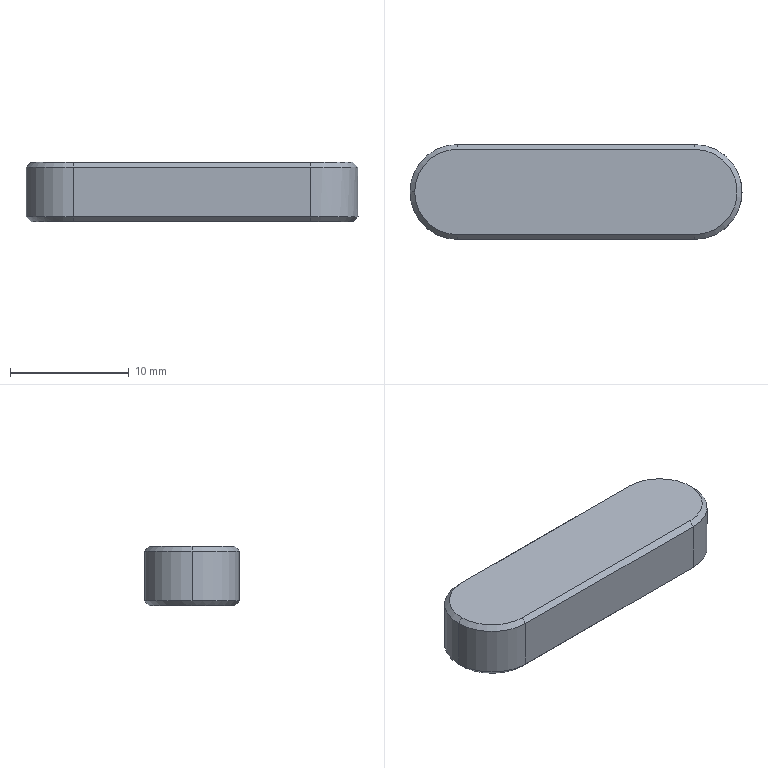Part | SolidWorks | features BaseBody 1 | 1 solid | 17 faces | box 28 x 8 x 5 mm | volume 1041 mm3 | plane 8 | cone 6 | cylinder 3 | commonest cylinder face diameters 8 x3
STEP:
#1=CARTESIAN_POINT('',(24.,-3.6,-3.));
#2=VERTEX_POINT('',#1);
#3=CARTESIAN_POINT('',(27.6,0.,-3.));
#4=VERTEX_POINT('',#3);
#5=CARTESIAN_POINT('',(24.,0.,-3.));
#6=DIRECTION('',(0.,0.,1.));
#7=DIRECTION('',(1.,0.,0.));
#8=AXIS2_PLACEMENT_3D('',#5,#6,#7);
#9=CIRCLE('',#8,3.6);
#10=EDGE_CURVE('',#2,#4,#9,.T.);
#11=ORIENTED_EDGE('',*,*,#10,.T.);
#12=CARTESIAN_POINT('',(28.,0.,-2.6));
#13=VERTEX_POINT('',#12);
#14=CARTESIAN_POINT('',(28.,0.,-2.6));
#15=DIRECTION('',(0.7071,0.,0.7071));
#16=VECTOR('',#15,1000.);
#17=LINE('',#14,#16);
#18=EDGE_CURVE('',#4,#13,#17,.T.);
#19=ORIENTED_EDGE('',*,*,#18,.T.);
#20=CARTESIAN_POINT('',(24.,-4.,-2.6));
#21=VERTEX_POINT('',#20);
#22=CARTESIAN_POINT('',(24.,0.,-2.6));
#23=DIRECTION('',(0.,0.,-1.));
#24=DIRECTION('',(0.,1.,0.));
#25=AXIS2_PLACEMENT_3D('',#22,#23,#24);
#26=CIRCLE('',#25,4.);
#27=EDGE_CURVE('',#13,#21,#26,.T.);
#28=ORIENTED_EDGE('',*,*,#27,.T.);
#29=CARTESIAN_POINT('',(24.,-3.8,-2.8));
#30=DIRECTION('',(0.,-0.7071,0.7071));
#31=VECTOR('',#30,1000.);
#32=LINE('',#29,#31);
#33=EDGE_CURVE('',#2,#21,#32,.T.);
#34=ORIENTED_EDGE('',*,*,#33,.F.);
#35=EDGE_LOOP('',(#11,#19,#28,#34));
#36=FACE_OUTER_BOUND('',#35,.T.);
#37=CARTESIAN_POINT('',(24.,0.,-2.6));
#38=DIRECTION('',(0.,0.,1.));
#39=DIRECTION('',(1.,0.,0.));
#40=AXIS2_PLACEMENT_3D('',#37,#38,#39);
#41=CONICAL_SURFACE('',#40,4.,0.7854);
#42=ADVANCED_FACE('',(#36),#41,.T.);
#43=CARTESIAN_POINT('',(4.,-4.,1.6));
#44=VERTEX_POINT('',#43);
#45=CARTESIAN_POINT('',(0.,0.,1.6));
#46=VERTEX_POINT('',#45);
#47=CARTESIAN_POINT('',(4.,0.,1.6));
#48=DIRECTION('',(0.,0.,-1.));
#49=DIRECTION('',(-1.,0.,0.));
#50=AXIS2_PLACEMENT_3D('',#47,#48,#49);
#51=CIRCLE('',#50,4.);
#52=EDGE_CURVE('',#44,#46,#51,.T.);
#53=ORIENTED_EDGE('',*,*,#52,.T.);
#54=CARTESIAN_POINT('',(0.,0.,-2.6));
#55=VERTEX_POINT('',#54);
#56=CARTESIAN_POINT('',(0.,0.,0.));
#57=DIRECTION('',(0.,0.,-1.));
#58=VECTOR('',#57,1000.);
#59=LINE('',#56,#58);
#60=EDGE_CURVE('',#46,#55,#59,.T.);
#61=ORIENTED_EDGE('',*,*,#60,.T.);
#62=CARTESIAN_POINT('',(4.,-4.,-2.6));
#63=VERTEX_POINT('',#62);
#64=CARTESIAN_POINT('',(4.,0.,-2.6));
#65=DIRECTION('',(0.,0.,-1.));
#66=DIRECTION('',(0.,-1.,0.));
#67=AXIS2_PLACEMENT_3D('',#64,#65,#66);
#68=CIRCLE('',#67,4.);
#69=EDGE_CURVE('',#63,#55,#68,.T.);
#70=ORIENTED_EDGE('',*,*,#69,.F.);
#71=CARTESIAN_POINT('',(4.,-4.,0.));
#72=DIRECTION('',(0.,0.,-1.));
#73=VECTOR('',#72,1000.);
#74=LINE('',#71,#73);
#75=EDGE_CURVE('',#44,#63,#74,.T.);
#76=ORIENTED_EDGE('',*,*,#75,.F.);
#77=EDGE_LOOP('',(#53,#61,#70,#76));
#78=FACE_OUTER_BOUND('',#77,.T.);
#79=CARTESIAN_POINT('',(4.,0.,0.));
#80=DIRECTION('',(0.,0.,-1.));
#81=DIRECTION('',(-1.,0.,0.));
#82=AXIS2_PLACEMENT_3D('',#79,#80,#81);
#83=CYLINDRICAL_SURFACE('',#82,4.);
#84=ADVANCED_FACE('',(#78),#83,.T.);
#85=CARTESIAN_POINT('',(4.,-3.6,2.));
#86=VERTEX_POINT('',#85);
#87=CARTESIAN_POINT('',(0.4,0.,2.));
#88=VERTEX_POINT('',#87);
#89=CARTESIAN_POINT('',(4.,0.,2.));
#90=DIRECTION('',(0.,0.,-1.));
#91=DIRECTION('',(-1.,0.,0.));
#92=AXIS2_PLACEMENT_3D('',#89,#90,#91);
#93=CIRCLE('',#92,3.6);
#94=EDGE_CURVE('',#86,#88,#93,.T.);
#95=ORIENTED_EDGE('',*,*,#94,.T.);
#96=CARTESIAN_POINT('',(0.,0.,1.6));
#97=DIRECTION('',(-0.7071,0.,-0.7071));
#98=VECTOR('',#97,1000.);
#99=LINE('',#96,#98);
#100=EDGE_CURVE('',#88,#46,#99,.T.);
#101=ORIENTED_EDGE('',*,*,#100,.T.);
#102=ORIENTED_EDGE('',*,*,#52,.F.);
#103=CARTESIAN_POINT('',(4.,-3.8,1.8));
#104=DIRECTION('',(0.,-0.7071,-0.7071));
#105=VECTOR('',#104,1000.);
#106=LINE('',#103,#105);
#107=EDGE_CURVE('',#86,#44,#106,.T.);
#108=ORIENTED_EDGE('',*,*,#107,.F.);
#109=EDGE_LOOP('',(#95,#101,#102,#108));
#110=FACE_OUTER_BOUND('',#109,.T.);
#111=CARTESIAN_POINT('',(4.,0.,1.6));
#112=DIRECTION('',(0.,0.,-1.));
#113=DIRECTION('',(-1.,0.,0.));
#114=AXIS2_PLACEMENT_3D('',#111,#112,#113);
#115=CONICAL_SURFACE('',#114,4.,0.7854);
#116=ADVANCED_FACE('',(#110),#115,.T.);
#117=CARTESIAN_POINT('',(4.,3.6,-3.));
#118=VERTEX_POINT('',#117);
#119=CARTESIAN_POINT('',(4.,-3.6,-3.));
#120=VERTEX_POINT('',#119);
#121=CARTESIAN_POINT('',(4.,0.,-3.));
#122=DIRECTION('',(0.,0.,1.));
#123=DIRECTION('',(1.,0.,0.));
#124=AXIS2_PLACEMENT_3D('',#121,#122,#123);
#125=CIRCLE('',#124,3.6);
#126=EDGE_CURVE('',#118,#120,#125,.T.);
#127=ORIENTED_EDGE('',*,*,#126,.F.);
#128=CARTESIAN_POINT('',(24.,3.6,-3.));
#129=VERTEX_POINT('',#128);
#130=CARTESIAN_POINT('',(14.,3.6,-3.));
#131=DIRECTION('',(-1.,0.,0.));
#132=VECTOR('',#131,1000.);
#133=LINE('',#130,#132);
#134=EDGE_CURVE('',#129,#118,#133,.T.);
#135=ORIENTED_EDGE('',*,*,#134,.F.);
#136=CARTESIAN_POINT('',(24.,0.,-3.));
#137=DIRECTION('',(0.,0.,1.));
#138=DIRECTION('',(1.,0.,0.));
#139=AXIS2_PLACEMENT_3D('',#136,#137,#138);
#140=CIRCLE('',#139,3.6);
#141=EDGE_CURVE('',#4,#129,#140,.T.);
#142=ORIENTED_EDGE('',*,*,#141,.F.);
#143=ORIENTED_EDGE('',*,*,#10,.F.);
#144=CARTESIAN_POINT('',(14.,-3.6,-3.));
#145=DIRECTION('',(1.,0.,0.));
#146=VECTOR('',#145,1000.);
#147=LINE('',#144,#146);
#148=EDGE_CURVE('',#120,#2,#147,.T.);
#149=ORIENTED_EDGE('',*,*,#148,.F.);
#150=EDGE_LOOP('',(#127,#135,#142,#143,#149));
#151=FACE_OUTER_BOUND('',#150,.T.);
#152=CARTESIAN_POINT('',(14.,0.,-3.));
#153=DIRECTION('',(0.,0.,1.));
#154=DIRECTION('',(1.,0.,0.));
#155=AXIS2_PLACEMENT_3D('',#152,#153,#154);
#156=PLANE('',#155);
#157=ADVANCED_FACE('',(#151),#156,.F.);
#158=CARTESIAN_POINT('',(4.,-3.8,-2.8));
#159=DIRECTION('',(0.,0.7071,-0.7071));
#160=VECTOR('',#159,1000.);
#161=LINE('',#158,#160);
#162=EDGE_CURVE('',#63,#120,#161,.T.);
#163=ORIENTED_EDGE('',*,*,#162,.T.);
#164=ORIENTED_EDGE('',*,*,#148,.T.);
#165=ORIENTED_EDGE('',*,*,#33,.T.);
#166=CARTESIAN_POINT('',(9.,-4.,-2.6));
#167=DIRECTION('',(-1.,0.,0.));
#168=VECTOR('',#167,1000.);
#169=LINE('',#166,#168);
#170=EDGE_CURVE('',#21,#63,#169,.T.);
#171=ORIENTED_EDGE('',*,*,#170,.T.);
#172=EDGE_LOOP('',(#163,#164,#165,#171));
#173=FACE_OUTER_BOUND('',#172,.T.);
#174=CARTESIAN_POINT('',(9.,-3.8,-2.8));
#175=DIRECTION('',(0.,-0.7071,-0.7071));
#176=DIRECTION('',(0.,0.7071,-0.7071));
#177=AXIS2_PLACEMENT_3D('',#174,#175,#176);
#178=PLANE('',#177);
#179=ADVANCED_FACE('',(#173),#178,.T.);
#180=ORIENTED_EDGE('',*,*,#162,.F.);
#181=ORIENTED_EDGE('',*,*,#69,.T.);
#182=CARTESIAN_POINT('',(4.,4.,-2.6));
#183=VERTEX_POINT('',#182);
#184=CARTESIAN_POINT('',(4.,0.,-2.6));
#185=DIRECTION('',(0.,0.,-1.));
#186=DIRECTION('',(0.,-1.,0.));
#187=AXIS2_PLACEMENT_3D('',#184,#185,#186);
#188=CIRCLE('',#187,4.);
#189=EDGE_CURVE('',#55,#183,#188,.T.);
#190=ORIENTED_EDGE('',*,*,#189,.T.);
#191=CARTESIAN_POINT('',(4.,499000.,498993.4));
#192=DIRECTION('',(0.,-0.7071,-0.7071));
#193=VECTOR('',#192,1000.);
#194=LINE('',#191,#193);
#195=EDGE_CURVE('',#183,#118,#194,.T.);
#196=ORIENTED_EDGE('',*,*,#195,.T.);
#197=ORIENTED_EDGE('',*,*,#126,.T.);
#198=EDGE_LOOP('',(#180,#181,#190,#196,#197));
#199=FACE_OUTER_BOUND('',#198,.T.);
#200=CARTESIAN_POINT('',(4.,0.,-2.6));
#201=DIRECTION('',(0.,0.,1.));
#202=DIRECTION('',(1.,0.,0.));
#203=AXIS2_PLACEMENT_3D('',#200,#201,#202);
#204=CONICAL_SURFACE('',#203,4.,0.7854);
#205=ADVANCED_FACE('',(#199),#204,.T.);
#206=ORIENTED_EDGE('',*,*,#195,.F.);
#207=CARTESIAN_POINT('',(24.,4.,-2.6));
#208=VERTEX_POINT('',#207);
#209=CARTESIAN_POINT('',(19.,4.,-2.6));
#210=DIRECTION('',(1.,0.,0.));
#211=VECTOR('',#210,1000.);
#212=LINE('',#209,#211);
#213=EDGE_CURVE('',#183,#208,#212,.T.);
#214=ORIENTED_EDGE('',*,*,#213,.T.);
#215=CARTESIAN_POINT('',(24.,3.8,-2.8));
#216=DIRECTION('',(0.,-0.7071,-0.7071));
#217=VECTOR('',#216,1000.);
#218=LINE('',#215,#217);
#219=EDGE_CURVE('',#208,#129,#218,.T.);
#220=ORIENTED_EDGE('',*,*,#219,.T.);
#221=ORIENTED_EDGE('',*,*,#134,.T.);
#222=EDGE_LOOP('',(#206,#214,#220,#221));
#223=FACE_OUTER_BOUND('',#222,.T.);
#224=CARTESIAN_POINT('',(19.,3.8,-2.8));
#225=DIRECTION('',(0.,0.7071,-0.7071));
#226=DIRECTION('',(0.,0.7071,0.7071));
#227=AXIS2_PLACEMENT_3D('',#224,#225,#226);
#228=PLANE('',#227);
#229=ADVANCED_FACE('',(#223),#228,.T.);
#230=ORIENTED_EDGE('',*,*,#18,.F.);
#231=ORIENTED_EDGE('',*,*,#141,.T.);
#232=ORIENTED_EDGE('',*,*,#219,.F.);
#233=CARTESIAN_POINT('',(24.,0.,-2.6));
#234=DIRECTION('',(0.,0.,-1.));
#235=DIRECTION('',(0.,1.,0.));
#236=AXIS2_PLACEMENT_3D('',#233,#234,#235);
#237=CIRCLE('',#236,4.);
#238=EDGE_CURVE('',#208,#13,#237,.T.);
#239=ORIENTED_EDGE('',*,*,#238,.T.);
#240=EDGE_LOOP('',(#230,#231,#232,#239));
#241=FACE_OUTER_BOUND('',#240,.T.);
#242=CARTESIAN_POINT('',(24.,0.,-2.6));
#243=DIRECTION('',(0.,0.,1.));
#244=DIRECTION('',(1.,0.,0.));
#245=AXIS2_PLACEMENT_3D('',#242,#243,#244);
#246=CONICAL_SURFACE('',#245,4.,0.7854);
#247=ADVANCED_FACE('',(#241),#246,.T.);
#248=CARTESIAN_POINT('',(24.,-4.,1.6));
#249=VERTEX_POINT('',#248);
#250=CARTESIAN_POINT('',(4.,-4.,1.6));
#251=DIRECTION('',(-1.,0.,0.));
#252=VECTOR('',#251,1000.);
#253=LINE('',#250,#252);
#254=EDGE_CURVE('',#249,#44,#253,.T.);
#255=ORIENTED_EDGE('',*,*,#254,.T.);
#256=ORIENTED_EDGE('',*,*,#75,.T.);
#257=ORIENTED_EDGE('',*,*,#170,.F.);
#258=CARTESIAN_POINT('',(24.,-4.,0.));
#259=DIRECTION('',(0.,0.,1.));
#260=VECTOR('',#259,1000.);
#261=LINE('',#258,#260);
#262=EDGE_CURVE('',#21,#249,#261,.T.);
#263=ORIENTED_EDGE('',*,*,#262,.T.);
#264=EDGE_LOOP('',(#255,#256,#257,#263));
#265=FACE_OUTER_BOUND('',#264,.T.);
#266=CARTESIAN_POINT('',(4.,-4.,0.));
#267=DIRECTION('',(0.,-1.,0.));
#268=DIRECTION('',(1.,0.,0.));
#269=AXIS2_PLACEMENT_3D('',#266,#267,#268);
#270=PLANE('',#269);
#271=ADVANCED_FACE('',(#265),#270,.T.);
#272=ORIENTED_EDGE('',*,*,#60,.F.);
#273=CARTESIAN_POINT('',(4.,4.,1.6));
#274=VERTEX_POINT('',#273);
#275=CARTESIAN_POINT('',(4.,0.,1.6));
#276=DIRECTION('',(0.,0.,-1.));
#277=DIRECTION('',(-1.,0.,0.));
#278=AXIS2_PLACEMENT_3D('',#275,#276,#277);
#279=CIRCLE('',#278,4.);
#280=EDGE_CURVE('',#46,#274,#279,.T.);
#281=ORIENTED_EDGE('',*,*,#280,.T.);
#282=CARTESIAN_POINT('',(4.,4.,0.));
#283=DIRECTION('',(0.,0.,-1.));
#284=VECTOR('',#283,1000.);
#285=LINE('',#282,#284);
#286=EDGE_CURVE('',#274,#183,#285,.T.);
#287=ORIENTED_EDGE('',*,*,#286,.T.);
#288=ORIENTED_EDGE('',*,*,#189,.F.);
#289=EDGE_LOOP('',(#272,#281,#287,#288));
#290=FACE_OUTER_BOUND('',#289,.T.);
#291=CARTESIAN_POINT('',(4.,0.,0.));
#292=DIRECTION('',(0.,0.,-1.));
#293=DIRECTION('',(-1.,0.,0.));
#294=AXIS2_PLACEMENT_3D('',#291,#292,#293);
#295=CYLINDRICAL_SURFACE('',#294,4.);
#296=ADVANCED_FACE('',(#290),#295,.T.);
#297=CARTESIAN_POINT('',(24.,4.,1.6));
#298=VERTEX_POINT('',#297);
#299=CARTESIAN_POINT('',(24.,4.,1.6));
#300=DIRECTION('',(1.,0.,0.));
#301=VECTOR('',#300,1000.);
#302=LINE('',#299,#301);
#303=EDGE_CURVE('',#274,#298,#302,.T.);
#304=ORIENTED_EDGE('',*,*,#303,.T.);
#305=CARTESIAN_POINT('',(24.,4.,0.));
#306=DIRECTION('',(0.,0.,-1.));
#307=VECTOR('',#306,1000.);
#308=LINE('',#305,#307);
#309=EDGE_CURVE('',#298,#208,#308,.T.);
#310=ORIENTED_EDGE('',*,*,#309,.T.);
#311=ORIENTED_EDGE('',*,*,#213,.F.);
#312=ORIENTED_EDGE('',*,*,#286,.F.);
#313=EDGE_LOOP('',(#304,#310,#311,#312));
#314=FACE_OUTER_BOUND('',#313,.T.);
#315=CARTESIAN_POINT('',(24.,4.,0.));
#316=DIRECTION('',(0.,1.,0.));
#317=DIRECTION('',(0.,0.,1.));
#318=AXIS2_PLACEMENT_3D('',#315,#316,#317);
#319=PLANE('',#318);
#320=ADVANCED_FACE('',(#314),#319,.T.);
#321=CARTESIAN_POINT('',(24.,0.,1.6));
#322=DIRECTION('',(0.,0.,-1.));
#323=DIRECTION('',(-1.,0.,0.));
#324=AXIS2_PLACEMENT_3D('',#321,#322,#323);
#325=CIRCLE('',#324,4.);
#326=EDGE_CURVE('',#298,#249,#325,.T.);
#327=ORIENTED_EDGE('',*,*,#326,.T.);
#328=ORIENTED_EDGE('',*,*,#262,.F.);
#329=ORIENTED_EDGE('',*,*,#27,.F.);
#330=ORIENTED_EDGE('',*,*,#238,.F.);
#331=ORIENTED_EDGE('',*,*,#309,.F.);
#332=EDGE_LOOP('',(#327,#328,#329,#330,#331));
#333=FACE_OUTER_BOUND('',#332,.T.);
#334=CARTESIAN_POINT('',(24.,0.,0.));
#335=DIRECTION('',(0.,0.,-1.));
#336=DIRECTION('',(-1.,0.,0.));
#337=AXIS2_PLACEMENT_3D('',#334,#335,#336);
#338=CYLINDRICAL_SURFACE('',#337,4.);
#339=ADVANCED_FACE('',(#333),#338,.T.);
#340=ORIENTED_EDGE('',*,*,#107,.T.);
#341=ORIENTED_EDGE('',*,*,#254,.F.);
#342=CARTESIAN_POINT('',(24.,-3.6,2.));
#343=VERTEX_POINT('',#342);
#344=CARTESIAN_POINT('',(24.,-3.8,1.8));
#345=DIRECTION('',(0.,0.7071,0.7071));
#346=VECTOR('',#345,1000.);
#347=LINE('',#344,#346);
#348=EDGE_CURVE('',#249,#343,#347,.T.);
#349=ORIENTED_EDGE('',*,*,#348,.T.);
#350=CARTESIAN_POINT('',(9.,-3.6,2.));
#351=DIRECTION('',(-1.,0.,0.));
#352=VECTOR('',#351,1000.);
#353=LINE('',#350,#352);
#354=EDGE_CURVE('',#343,#86,#353,.T.);
#355=ORIENTED_EDGE('',*,*,#354,.T.);
#356=EDGE_LOOP('',(#340,#341,#349,#355));
#357=FACE_OUTER_BOUND('',#356,.T.);
#358=CARTESIAN_POINT('',(9.,-3.8,1.8));
#359=DIRECTION('',(0.,-0.7071,0.7071));
#360=DIRECTION('',(0.,-0.7071,-0.7071));
#361=AXIS2_PLACEMENT_3D('',#358,#359,#360);
#362=PLANE('',#361);
#363=ADVANCED_FACE('',(#357),#362,.T.);
#364=ORIENTED_EDGE('',*,*,#100,.F.);
#365=CARTESIAN_POINT('',(4.,3.6,2.));
#366=VERTEX_POINT('',#365);
#367=CARTESIAN_POINT('',(4.,0.,2.));
#368=DIRECTION('',(0.,0.,-1.));
#369=DIRECTION('',(-1.,0.,0.));
#370=AXIS2_PLACEMENT_3D('',#367,#368,#369);
#371=CIRCLE('',#370,3.6);
#372=EDGE_CURVE('',#88,#366,#371,.T.);
#373=ORIENTED_EDGE('',*,*,#372,.T.);
#374=CARTESIAN_POINT('',(4.,499000.,-498994.4));
#375=DIRECTION('',(0.,0.7071,-0.7071));
#376=VECTOR('',#375,1000.);
#377=LINE('',#374,#376);
#378=EDGE_CURVE('',#366,#274,#377,.T.);
#379=ORIENTED_EDGE('',*,*,#378,.T.);
#380=ORIENTED_EDGE('',*,*,#280,.F.);
#381=EDGE_LOOP('',(#364,#373,#379,#380));
#382=FACE_OUTER_BOUND('',#381,.T.);
#383=CARTESIAN_POINT('',(4.,0.,1.6));
#384=DIRECTION('',(0.,0.,-1.));
#385=DIRECTION('',(-1.,0.,0.));
#386=AXIS2_PLACEMENT_3D('',#383,#384,#385);
#387=CONICAL_SURFACE('',#386,4.,0.7854);
#388=ADVANCED_FACE('',(#382),#387,.T.);
#389=ORIENTED_EDGE('',*,*,#378,.F.);
#390=CARTESIAN_POINT('',(24.,3.6,2.));
#391=VERTEX_POINT('',#390);
#392=CARTESIAN_POINT('',(19.,3.6,2.));
#393=DIRECTION('',(1.,0.,0.));
#394=VECTOR('',#393,1000.);
#395=LINE('',#392,#394);
#396=EDGE_CURVE('',#366,#391,#395,.T.);
#397=ORIENTED_EDGE('',*,*,#396,.T.);
#398=CARTESIAN_POINT('',(24.,3.8,1.8));
#399=DIRECTION('',(0.,0.7071,-0.7071));
#400=VECTOR('',#399,1000.);
#401=LINE('',#398,#400);
#402=EDGE_CURVE('',#391,#298,#401,.T.);
#403=ORIENTED_EDGE('',*,*,#402,.T.);
#404=ORIENTED_EDGE('',*,*,#303,.F.);
#405=EDGE_LOOP('',(#389,#397,#403,#404));
#406=FACE_OUTER_BOUND('',#405,.T.);
#407=CARTESIAN_POINT('',(19.,3.8,1.8));
#408=DIRECTION('',(0.,0.7071,0.7071));
#409=DIRECTION('',(0.,-0.7071,0.7071));
#410=AXIS2_PLACEMENT_3D('',#407,#408,#409);
#411=PLANE('',#410);
#412=ADVANCED_FACE('',(#406),#411,.T.);
#413=ORIENTED_EDGE('',*,*,#402,.F.);
#414=CARTESIAN_POINT('',(24.,0.,2.));
#415=DIRECTION('',(0.,0.,-1.));
#416=DIRECTION('',(-1.,0.,0.));
#417=AXIS2_PLACEMENT_3D('',#414,#415,#416);
#418=CIRCLE('',#417,3.6);
#419=EDGE_CURVE('',#391,#343,#418,.T.);
#420=ORIENTED_EDGE('',*,*,#419,.T.);
#421=ORIENTED_EDGE('',*,*,#348,.F.);
#422=ORIENTED_EDGE('',*,*,#326,.F.);
#423=EDGE_LOOP('',(#413,#420,#421,#422));
#424=FACE_OUTER_BOUND('',#423,.T.);
#425=CARTESIAN_POINT('',(24.,0.,1.6));
#426=DIRECTION('',(0.,0.,-1.));
#427=DIRECTION('',(-1.,0.,0.));
#428=AXIS2_PLACEMENT_3D('',#425,#426,#427);
#429=CONICAL_SURFACE('',#428,4.,0.7854);
#430=ADVANCED_FACE('',(#424),#429,.T.);
#431=ORIENTED_EDGE('',*,*,#419,.F.);
#432=ORIENTED_EDGE('',*,*,#396,.F.);
#433=ORIENTED_EDGE('',*,*,#372,.F.);
#434=ORIENTED_EDGE('',*,*,#94,.F.);
#435=ORIENTED_EDGE('',*,*,#354,.F.);
#436=EDGE_LOOP('',(#431,#432,#433,#434,#435));
#437=FACE_OUTER_BOUND('',#436,.T.);
#438=CARTESIAN_POINT('',(14.,0.,2.));
#439=DIRECTION('',(0.,0.,1.));
#440=DIRECTION('',(1.,0.,0.));
#441=AXIS2_PLACEMENT_3D('',#438,#439,#440);
#442=PLANE('',#441);
#443=ADVANCED_FACE('',(#437),#442,.T.);
#444=CLOSED_SHELL('',(#42,#84,#116,#157,#179,#205,#229,#247,#271,#296,#320,#339,#363,#388,#412,#430,#443));
#445=MANIFOLD_SOLID_BREP('',#444);
#446=CARTESIAN_POINT('',(0.,0.,0.));
#447=DIRECTION('',(0.,0.,1.));
#448=DIRECTION('',(1.,0.,0.));
#449=AXIS2_PLACEMENT_3D('',#446,#447,#448);
#450=(LENGTH_UNIT()NAMED_UNIT(*)SI_UNIT(.MILLI.,.METRE.));
#451=UNCERTAINTY_MEASURE_WITH_UNIT(LENGTH_MEASURE(0.00001),#450,'','');
#452=(NAMED_UNIT(*)PLANE_ANGLE_UNIT()SI_UNIT($,.RADIAN.));
#453=(NAMED_UNIT(*)SI_UNIT($,.STERADIAN.)SOLID_ANGLE_UNIT());
#454=(GEOMETRIC_REPRESENTATION_CONTEXT(3)GLOBAL_UNCERTAINTY_ASSIGNED_CONTEXT((#451))GLOBAL_UNIT_ASSIGNED_CONTEXT((#450,#452,#453))REPRESENTATION_CONTEXT('',''));
#455=ADVANCED_BREP_SHAPE_REPRESENTATION('',(#445,#449),#454);